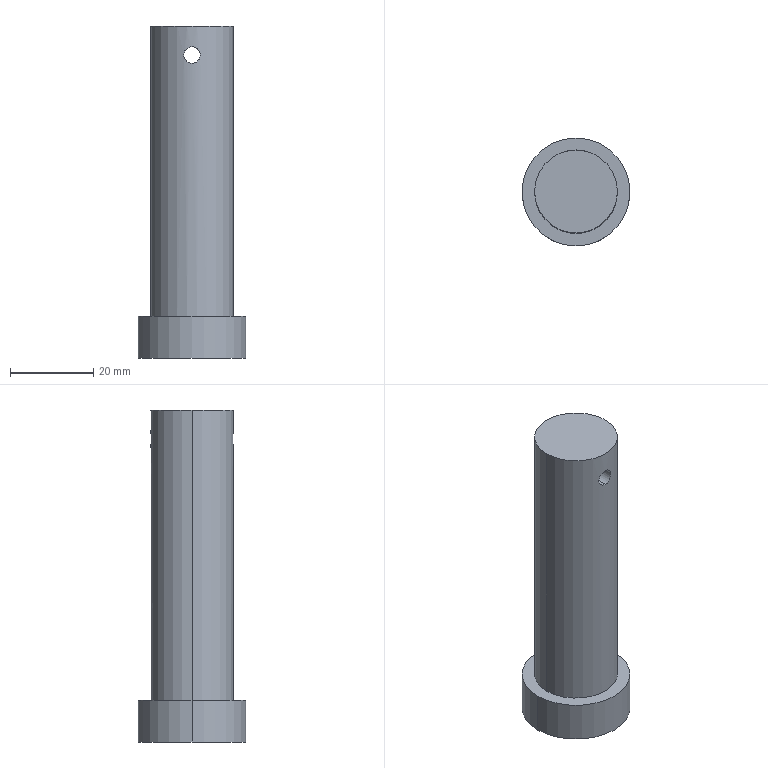Part | SolidWorks | features ICE 2, Extrusion 1 | 1 solid | 9 faces | box 26 x 26 x 80 mm | volume 27050 mm3 | cylinder 6 | plane 3 | commonest cylinder face diameters 4 x2 20 x2 26 x2
STEP:
#1=CARTESIAN_POINT('',(0.,-10.,61.));
#2=VERTEX_POINT('',#1);
#3=CARTESIAN_POINT('',(0.,-10.,65.));
#4=VERTEX_POINT('',#3);
#5=CARTESIAN_POINT('',(0.,-10.,61.));
#6=CARTESIAN_POINT('',(-0.2614,-10.,61.));
#7=CARTESIAN_POINT('',(-0.5251,-9.989,61.053));
#8=CARTESIAN_POINT('',(-0.8863,-9.961,61.202));
#9=CARTESIAN_POINT('',(-1.003,-9.95,61.265));
#10=CARTESIAN_POINT('',(-1.221,-9.926,61.41));
#11=CARTESIAN_POINT('',(-1.321,-9.913,61.493));
#12=CARTESIAN_POINT('',(-1.506,-9.886,61.677));
#13=CARTESIAN_POINT('',(-1.59,-9.873,61.78));
#14=CARTESIAN_POINT('',(-1.735,-9.849,61.996));
#15=CARTESIAN_POINT('',(-1.796,-9.837,62.111));
#16=CARTESIAN_POINT('',(-1.948,-9.809,62.475));
#17=CARTESIAN_POINT('',(-2.,-9.798,62.735));
#18=CARTESIAN_POINT('',(-2.,-9.798,63.131));
#19=CARTESIAN_POINT('',(-1.987,-9.801,63.261));
#20=CARTESIAN_POINT('',(-1.936,-9.811,63.517));
#21=CARTESIAN_POINT('',(-1.898,-9.818,63.645));
#22=CARTESIAN_POINT('',(-1.798,-9.837,63.887));
#23=CARTESIAN_POINT('',(-1.736,-9.848,64.001));
#24=CARTESIAN_POINT('',(-1.591,-9.873,64.219));
#25=CARTESIAN_POINT('',(-1.507,-9.886,64.321));
#26=CARTESIAN_POINT('',(-1.231,-9.926,64.597));
#27=CARTESIAN_POINT('',(-1.009,-9.952,64.746));
#28=CARTESIAN_POINT('',(-0.6482,-9.98,64.897));
#29=CARTESIAN_POINT('',(-0.5213,-9.987,64.935));
#30=CARTESIAN_POINT('',(-0.2632,-9.997,64.987));
#31=CARTESIAN_POINT('',(-0.1325,-10.,65.));
#32=CARTESIAN_POINT('',(0.,-10.,65.));
#33=B_SPLINE_CURVE_WITH_KNOTS('',3,(#5,#6,#7,#8,#9,#10,#11,#12,#13,#14,#15,#16,#17,#18,#19,#20,#21,#22,#23,#24,#25,#26,#27,#28,#29,#30,#31,#32),.UNSPECIFIED.,.F.,.F.,(4,2,2,2,2,2,2,2,2,2,2,2,2,4),(0.006269,0.007052,0.007444,0.007836,0.008227,0.008619,0.009402,0.009794,0.01019,0.01058,0.01097,0.01175,0.01214,0.01254),.UNSPECIFIED.);
#34=EDGE_CURVE('',#2,#4,#33,.T.);
#35=ORIENTED_EDGE('',*,*,#34,.F.);
#36=CARTESIAN_POINT('',(0.,10.,61.));
#37=VERTEX_POINT('',#36);
#38=CARTESIAN_POINT('',(0.,-13.,61.));
#39=DIRECTION('',(0.,1.,0.));
#40=VECTOR('',#39,1000.);
#41=LINE('',#38,#40);
#42=EDGE_CURVE('',#2,#37,#41,.T.);
#43=ORIENTED_EDGE('',*,*,#42,.T.);
#44=CARTESIAN_POINT('',(0.,10.,65.));
#45=VERTEX_POINT('',#44);
#46=CARTESIAN_POINT('',(0.,10.,65.));
#47=CARTESIAN_POINT('',(-0.1325,10.,65.));
#48=CARTESIAN_POINT('',(-0.2627,9.997,64.987));
#49=CARTESIAN_POINT('',(-0.5188,9.987,64.936));
#50=CARTESIAN_POINT('',(-0.646,9.98,64.897));
#51=CARTESIAN_POINT('',(-0.8881,9.961,64.797));
#52=CARTESIAN_POINT('',(-1.003,9.95,64.735));
#53=CARTESIAN_POINT('',(-1.22,9.926,64.59));
#54=CARTESIAN_POINT('',(-1.323,9.913,64.506));
#55=CARTESIAN_POINT('',(-1.599,9.873,64.23));
#56=CARTESIAN_POINT('',(-1.747,9.847,64.007));
#57=CARTESIAN_POINT('',(-1.947,9.809,63.526));
#58=CARTESIAN_POINT('',(-2.,9.798,63.262));
#59=CARTESIAN_POINT('',(-2.,9.798,62.87));
#60=CARTESIAN_POINT('',(-1.987,9.801,62.737));
#61=CARTESIAN_POINT('',(-1.936,9.811,62.48));
#62=CARTESIAN_POINT('',(-1.898,9.818,62.355));
#63=CARTESIAN_POINT('',(-1.747,9.847,61.992));
#64=CARTESIAN_POINT('',(-1.6,9.873,61.772));
#65=CARTESIAN_POINT('',(-1.321,9.913,61.493));
#66=CARTESIAN_POINT('',(-1.22,9.926,61.41));
#67=CARTESIAN_POINT('',(-1.004,9.95,61.265));
#68=CARTESIAN_POINT('',(-0.887,9.961,61.203));
#69=CARTESIAN_POINT('',(-0.6452,9.98,61.102));
#70=CARTESIAN_POINT('',(-0.5206,9.987,61.064));
#71=CARTESIAN_POINT('',(-0.2635,9.997,61.013));
#72=CARTESIAN_POINT('',(-0.1307,10.,61.));
#73=CARTESIAN_POINT('',(0.,10.,61.));
#74=B_SPLINE_CURVE_WITH_KNOTS('',3,(#46,#47,#48,#49,#50,#51,#52,#53,#54,#55,#56,#57,#58,#59,#60,#61,#62,#63,#64,#65,#66,#67,#68,#69,#70,#71,#72,#73),.UNSPECIFIED.,.F.,.F.,(4,2,2,2,2,2,2,2,2,2,2,2,2,4),(0.,0.0003918,0.0007836,0.001175,0.001567,0.002351,0.003134,0.003526,0.003918,0.004702,0.005093,0.005485,0.005877,0.006269),.UNSPECIFIED.);
#75=EDGE_CURVE('',#45,#37,#74,.T.);
#76=ORIENTED_EDGE('',*,*,#75,.F.);
#77=CARTESIAN_POINT('',(0.,-13.,65.));
#78=DIRECTION('',(0.,1.,0.));
#79=VECTOR('',#78,1000.);
#80=LINE('',#77,#79);
#81=EDGE_CURVE('',#4,#45,#80,.T.);
#82=ORIENTED_EDGE('',*,*,#81,.F.);
#83=EDGE_LOOP('',(#35,#43,#76,#82));
#84=FACE_OUTER_BOUND('',#83,.T.);
#85=CARTESIAN_POINT('',(0.,-13.,63.));
#86=DIRECTION('',(0.,1.,0.));
#87=DIRECTION('',(0.,0.,1.));
#88=AXIS2_PLACEMENT_3D('',#85,#86,#87);
#89=CYLINDRICAL_SURFACE('',#88,2.);
#90=ADVANCED_FACE('',(#84),#89,.F.);
#91=CARTESIAN_POINT('',(-13.,0.,-10.));
#92=VERTEX_POINT('',#91);
#93=CARTESIAN_POINT('',(13.,0.,-10.));
#94=VERTEX_POINT('',#93);
#95=CARTESIAN_POINT('',(0.,0.,-10.));
#96=DIRECTION('',(0.,0.,-1.));
#97=DIRECTION('',(-1.,0.,0.));
#98=AXIS2_PLACEMENT_3D('',#95,#96,#97);
#99=CIRCLE('',#98,13.);
#100=EDGE_CURVE('',#92,#94,#99,.T.);
#101=ORIENTED_EDGE('',*,*,#100,.F.);
#102=CARTESIAN_POINT('',(-13.,0.,0.));
#103=VERTEX_POINT('',#102);
#104=CARTESIAN_POINT('',(-13.,0.,-10.));
#105=DIRECTION('',(0.,0.,1.));
#106=VECTOR('',#105,1000.);
#107=LINE('',#104,#106);
#108=EDGE_CURVE('',#92,#103,#107,.T.);
#109=ORIENTED_EDGE('',*,*,#108,.T.);
#110=CARTESIAN_POINT('',(13.,0.,0.));
#111=VERTEX_POINT('',#110);
#112=CARTESIAN_POINT('',(0.,0.,0.));
#113=DIRECTION('',(0.,0.,-1.));
#114=DIRECTION('',(-1.,0.,0.));
#115=AXIS2_PLACEMENT_3D('',#112,#113,#114);
#116=CIRCLE('',#115,13.);
#117=EDGE_CURVE('',#103,#111,#116,.T.);
#118=ORIENTED_EDGE('',*,*,#117,.T.);
#119=CARTESIAN_POINT('',(13.,0.,-10.));
#120=DIRECTION('',(0.,0.,1.));
#121=VECTOR('',#120,1000.);
#122=LINE('',#119,#121);
#123=EDGE_CURVE('',#94,#111,#122,.T.);
#124=ORIENTED_EDGE('',*,*,#123,.F.);
#125=EDGE_LOOP('',(#101,#109,#118,#124));
#126=FACE_OUTER_BOUND('',#125,.T.);
#127=CARTESIAN_POINT('',(0.,0.,-10.));
#128=DIRECTION('',(0.,0.,1.));
#129=DIRECTION('',(1.,0.,0.));
#130=AXIS2_PLACEMENT_3D('',#127,#128,#129);
#131=CYLINDRICAL_SURFACE('',#130,13.);
#132=ADVANCED_FACE('',(#126),#131,.T.);
#133=ORIENTED_EDGE('',*,*,#75,.T.);
#134=CARTESIAN_POINT('',(0.,10.,61.));
#135=CARTESIAN_POINT('',(0.2614,10.,61.));
#136=CARTESIAN_POINT('',(0.5251,9.989,61.053));
#137=CARTESIAN_POINT('',(0.8863,9.961,61.202));
#138=CARTESIAN_POINT('',(1.003,9.95,61.265));
#139=CARTESIAN_POINT('',(1.221,9.926,61.41));
#140=CARTESIAN_POINT('',(1.321,9.913,61.493));
#141=CARTESIAN_POINT('',(1.506,9.886,61.677));
#142=CARTESIAN_POINT('',(1.59,9.873,61.78));
#143=CARTESIAN_POINT('',(1.735,9.849,61.996));
#144=CARTESIAN_POINT('',(1.796,9.837,62.111));
#145=CARTESIAN_POINT('',(1.948,9.809,62.475));
#146=CARTESIAN_POINT('',(2.,9.798,62.735));
#147=CARTESIAN_POINT('',(2.,9.798,63.131));
#148=CARTESIAN_POINT('',(1.987,9.801,63.261));
#149=CARTESIAN_POINT('',(1.936,9.811,63.517));
#150=CARTESIAN_POINT('',(1.898,9.818,63.645));
#151=CARTESIAN_POINT('',(1.798,9.837,63.887));
#152=CARTESIAN_POINT('',(1.736,9.848,64.001));
#153=CARTESIAN_POINT('',(1.591,9.873,64.219));
#154=CARTESIAN_POINT('',(1.507,9.886,64.321));
#155=CARTESIAN_POINT('',(1.231,9.926,64.597));
#156=CARTESIAN_POINT('',(1.009,9.952,64.746));
#157=CARTESIAN_POINT('',(0.6482,9.98,64.897));
#158=CARTESIAN_POINT('',(0.5213,9.987,64.935));
#159=CARTESIAN_POINT('',(0.2632,9.997,64.987));
#160=CARTESIAN_POINT('',(0.1325,10.,65.));
#161=CARTESIAN_POINT('',(0.,10.,65.));
#162=B_SPLINE_CURVE_WITH_KNOTS('',3,(#134,#135,#136,#137,#138,#139,#140,#141,#142,#143,#144,#145,#146,#147,#148,#149,#150,#151,#152,#153,#154,#155,#156,#157,#158,#159,#160,#161),.UNSPECIFIED.,.F.,.F.,(4,2,2,2,2,2,2,2,2,2,2,2,2,4),(0.006269,0.007052,0.007444,0.007836,0.008227,0.008619,0.009402,0.009794,0.01019,0.01058,0.01097,0.01175,0.01214,0.01254),.UNSPECIFIED.);
#163=EDGE_CURVE('',#37,#45,#162,.T.);
#164=ORIENTED_EDGE('',*,*,#163,.T.);
#165=EDGE_LOOP('',(#133,#164));
#166=FACE_BOUND('',#165,.T.);
#167=CARTESIAN_POINT('',(10.,0.,70.));
#168=VERTEX_POINT('',#167);
#169=CARTESIAN_POINT('',(-10.,0.,70.));
#170=VERTEX_POINT('',#169);
#171=CARTESIAN_POINT('',(0.,0.,70.));
#172=DIRECTION('',(0.,0.,1.));
#173=DIRECTION('',(1.,0.,0.));
#174=AXIS2_PLACEMENT_3D('',#171,#172,#173);
#175=CIRCLE('',#174,10.);
#176=EDGE_CURVE('',#168,#170,#175,.T.);
#177=ORIENTED_EDGE('',*,*,#176,.F.);
#178=CARTESIAN_POINT('',(10.,0.,0.));
#179=VERTEX_POINT('',#178);
#180=CARTESIAN_POINT('',(10.,0.,70.));
#181=DIRECTION('',(0.,0.,-1.));
#182=VECTOR('',#181,1000.);
#183=LINE('',#180,#182);
#184=EDGE_CURVE('',#168,#179,#183,.T.);
#185=ORIENTED_EDGE('',*,*,#184,.T.);
#186=CARTESIAN_POINT('',(-10.,0.,0.));
#187=VERTEX_POINT('',#186);
#188=CARTESIAN_POINT('',(0.,0.,0.));
#189=DIRECTION('',(0.,0.,-1.));
#190=DIRECTION('',(-1.,0.,0.));
#191=AXIS2_PLACEMENT_3D('',#188,#189,#190);
#192=CIRCLE('',#191,10.);
#193=EDGE_CURVE('',#187,#179,#192,.T.);
#194=ORIENTED_EDGE('',*,*,#193,.F.);
#195=CARTESIAN_POINT('',(-10.,0.,70.));
#196=DIRECTION('',(0.,0.,-1.));
#197=VECTOR('',#196,1000.);
#198=LINE('',#195,#197);
#199=EDGE_CURVE('',#170,#187,#198,.T.);
#200=ORIENTED_EDGE('',*,*,#199,.F.);
#201=EDGE_LOOP('',(#177,#185,#194,#200));
#202=FACE_OUTER_BOUND('',#201,.T.);
#203=CARTESIAN_POINT('',(0.,0.,70.));
#204=DIRECTION('',(0.,0.,-1.));
#205=DIRECTION('',(-1.,0.,0.));
#206=AXIS2_PLACEMENT_3D('',#203,#204,#205);
#207=CYLINDRICAL_SURFACE('',#206,10.);
#208=ADVANCED_FACE('',(#166,#202),#207,.T.);
#209=ORIENTED_EDGE('',*,*,#184,.F.);
#210=CARTESIAN_POINT('',(0.,0.,70.));
#211=DIRECTION('',(0.,0.,1.));
#212=DIRECTION('',(1.,0.,0.));
#213=AXIS2_PLACEMENT_3D('',#210,#211,#212);
#214=CIRCLE('',#213,10.);
#215=EDGE_CURVE('',#170,#168,#214,.T.);
#216=ORIENTED_EDGE('',*,*,#215,.F.);
#217=ORIENTED_EDGE('',*,*,#199,.T.);
#218=CARTESIAN_POINT('',(0.,0.,0.));
#219=DIRECTION('',(0.,0.,-1.));
#220=DIRECTION('',(-1.,0.,0.));
#221=AXIS2_PLACEMENT_3D('',#218,#219,#220);
#222=CIRCLE('',#221,10.);
#223=EDGE_CURVE('',#179,#187,#222,.T.);
#224=ORIENTED_EDGE('',*,*,#223,.F.);
#225=EDGE_LOOP('',(#209,#216,#217,#224));
#226=FACE_OUTER_BOUND('',#225,.T.);
#227=CARTESIAN_POINT('',(0.,-10.,65.));
#228=CARTESIAN_POINT('',(0.1325,-10.,65.));
#229=CARTESIAN_POINT('',(0.2627,-9.997,64.987));
#230=CARTESIAN_POINT('',(0.5188,-9.987,64.936));
#231=CARTESIAN_POINT('',(0.646,-9.98,64.897));
#232=CARTESIAN_POINT('',(0.8881,-9.961,64.797));
#233=CARTESIAN_POINT('',(1.003,-9.95,64.735));
#234=CARTESIAN_POINT('',(1.22,-9.926,64.59));
#235=CARTESIAN_POINT('',(1.323,-9.913,64.506));
#236=CARTESIAN_POINT('',(1.599,-9.873,64.23));
#237=CARTESIAN_POINT('',(1.747,-9.847,64.007));
#238=CARTESIAN_POINT('',(1.947,-9.809,63.526));
#239=CARTESIAN_POINT('',(2.,-9.798,63.262));
#240=CARTESIAN_POINT('',(2.,-9.798,62.87));
#241=CARTESIAN_POINT('',(1.987,-9.801,62.737));
#242=CARTESIAN_POINT('',(1.936,-9.811,62.48));
#243=CARTESIAN_POINT('',(1.898,-9.818,62.355));
#244=CARTESIAN_POINT('',(1.747,-9.847,61.992));
#245=CARTESIAN_POINT('',(1.6,-9.873,61.772));
#246=CARTESIAN_POINT('',(1.321,-9.913,61.493));
#247=CARTESIAN_POINT('',(1.22,-9.926,61.41));
#248=CARTESIAN_POINT('',(1.004,-9.95,61.265));
#249=CARTESIAN_POINT('',(0.887,-9.961,61.203));
#250=CARTESIAN_POINT('',(0.6452,-9.98,61.102));
#251=CARTESIAN_POINT('',(0.5206,-9.987,61.064));
#252=CARTESIAN_POINT('',(0.2635,-9.997,61.013));
#253=CARTESIAN_POINT('',(0.1307,-10.,61.));
#254=CARTESIAN_POINT('',(0.,-10.,61.));
#255=B_SPLINE_CURVE_WITH_KNOTS('',3,(#227,#228,#229,#230,#231,#232,#233,#234,#235,#236,#237,#238,#239,#240,#241,#242,#243,#244,#245,#246,#247,#248,#249,#250,#251,#252,#253,#254),.UNSPECIFIED.,.F.,.F.,(4,2,2,2,2,2,2,2,2,2,2,2,2,4),(0.,0.0003918,0.0007836,0.001175,0.001567,0.002351,0.003134,0.003526,0.003918,0.004702,0.005093,0.005485,0.005877,0.006269),.UNSPECIFIED.);
#256=EDGE_CURVE('',#4,#2,#255,.T.);
#257=ORIENTED_EDGE('',*,*,#256,.T.);
#258=ORIENTED_EDGE('',*,*,#34,.T.);
#259=EDGE_LOOP('',(#257,#258));
#260=FACE_BOUND('',#259,.T.);
#261=CARTESIAN_POINT('',(0.,0.,70.));
#262=DIRECTION('',(0.,0.,-1.));
#263=DIRECTION('',(-1.,0.,0.));
#264=AXIS2_PLACEMENT_3D('',#261,#262,#263);
#265=CYLINDRICAL_SURFACE('',#264,10.);
#266=ADVANCED_FACE('',(#226,#260),#265,.T.);
#267=ORIENTED_EDGE('',*,*,#215,.T.);
#268=ORIENTED_EDGE('',*,*,#176,.T.);
#269=EDGE_LOOP('',(#267,#268));
#270=FACE_OUTER_BOUND('',#269,.T.);
#271=CARTESIAN_POINT('',(0.,0.,70.));
#272=DIRECTION('',(0.,0.,1.));
#273=DIRECTION('',(1.,0.,0.));
#274=AXIS2_PLACEMENT_3D('',#271,#272,#273);
#275=PLANE('',#274);
#276=ADVANCED_FACE('',(#270),#275,.T.);
#277=ORIENTED_EDGE('',*,*,#108,.F.);
#278=CARTESIAN_POINT('',(0.,0.,-10.));
#279=DIRECTION('',(0.,0.,-1.));
#280=DIRECTION('',(-1.,0.,0.));
#281=AXIS2_PLACEMENT_3D('',#278,#279,#280);
#282=CIRCLE('',#281,13.);
#283=EDGE_CURVE('',#94,#92,#282,.T.);
#284=ORIENTED_EDGE('',*,*,#283,.F.);
#285=ORIENTED_EDGE('',*,*,#123,.T.);
#286=CARTESIAN_POINT('',(0.,0.,0.));
#287=DIRECTION('',(0.,0.,-1.));
#288=DIRECTION('',(-1.,0.,0.));
#289=AXIS2_PLACEMENT_3D('',#286,#287,#288);
#290=CIRCLE('',#289,13.);
#291=EDGE_CURVE('',#111,#103,#290,.T.);
#292=ORIENTED_EDGE('',*,*,#291,.T.);
#293=EDGE_LOOP('',(#277,#284,#285,#292));
#294=FACE_OUTER_BOUND('',#293,.T.);
#295=CARTESIAN_POINT('',(0.,0.,-10.));
#296=DIRECTION('',(0.,0.,1.));
#297=DIRECTION('',(1.,0.,0.));
#298=AXIS2_PLACEMENT_3D('',#295,#296,#297);
#299=CYLINDRICAL_SURFACE('',#298,13.);
#300=ADVANCED_FACE('',(#294),#299,.T.);
#301=ORIENTED_EDGE('',*,*,#283,.T.);
#302=ORIENTED_EDGE('',*,*,#100,.T.);
#303=EDGE_LOOP('',(#301,#302));
#304=FACE_OUTER_BOUND('',#303,.T.);
#305=CARTESIAN_POINT('',(0.,0.,-10.));
#306=DIRECTION('',(0.,0.,-1.));
#307=DIRECTION('',(-1.,0.,0.));
#308=AXIS2_PLACEMENT_3D('',#305,#306,#307);
#309=PLANE('',#308);
#310=ADVANCED_FACE('',(#304),#309,.T.);
#311=ORIENTED_EDGE('',*,*,#193,.T.);
#312=ORIENTED_EDGE('',*,*,#223,.T.);
#313=EDGE_LOOP('',(#311,#312));
#314=FACE_BOUND('',#313,.T.);
#315=ORIENTED_EDGE('',*,*,#291,.F.);
#316=ORIENTED_EDGE('',*,*,#117,.F.);
#317=EDGE_LOOP('',(#315,#316));
#318=FACE_OUTER_BOUND('',#317,.T.);
#319=CARTESIAN_POINT('',(0.,0.,0.));
#320=DIRECTION('',(0.,0.,-1.));
#321=DIRECTION('',(-1.,0.,0.));
#322=AXIS2_PLACEMENT_3D('',#319,#320,#321);
#323=PLANE('',#322);
#324=ADVANCED_FACE('',(#314,#318),#323,.F.);
#325=ORIENTED_EDGE('',*,*,#42,.F.);
#326=ORIENTED_EDGE('',*,*,#256,.F.);
#327=ORIENTED_EDGE('',*,*,#81,.T.);
#328=ORIENTED_EDGE('',*,*,#163,.F.);
#329=EDGE_LOOP('',(#325,#326,#327,#328));
#330=FACE_OUTER_BOUND('',#329,.T.);
#331=CARTESIAN_POINT('',(0.,-13.,63.));
#332=DIRECTION('',(0.,1.,0.));
#333=DIRECTION('',(0.,0.,1.));
#334=AXIS2_PLACEMENT_3D('',#331,#332,#333);
#335=CYLINDRICAL_SURFACE('',#334,2.);
#336=ADVANCED_FACE('',(#330),#335,.F.);
#337=CLOSED_SHELL('',(#90,#132,#208,#266,#276,#300,#310,#324,#336));
#338=MANIFOLD_SOLID_BREP('',#337);
#339=CARTESIAN_POINT('',(0.,0.,0.));
#340=DIRECTION('',(0.,0.,1.));
#341=DIRECTION('',(1.,0.,0.));
#342=AXIS2_PLACEMENT_3D('',#339,#340,#341);
#343=(LENGTH_UNIT()NAMED_UNIT(*)SI_UNIT(.MILLI.,.METRE.));
#344=UNCERTAINTY_MEASURE_WITH_UNIT(LENGTH_MEASURE(0.00001),#343,'','');
#345=(NAMED_UNIT(*)PLANE_ANGLE_UNIT()SI_UNIT($,.RADIAN.));
#346=(NAMED_UNIT(*)SI_UNIT($,.STERADIAN.)SOLID_ANGLE_UNIT());
#347=(GEOMETRIC_REPRESENTATION_CONTEXT(3)GLOBAL_UNCERTAINTY_ASSIGNED_CONTEXT((#344))GLOBAL_UNIT_ASSIGNED_CONTEXT((#343,#345,#346))REPRESENTATION_CONTEXT('',''));
#348=ADVANCED_BREP_SHAPE_REPRESENTATION('',(#338,#342),#347);